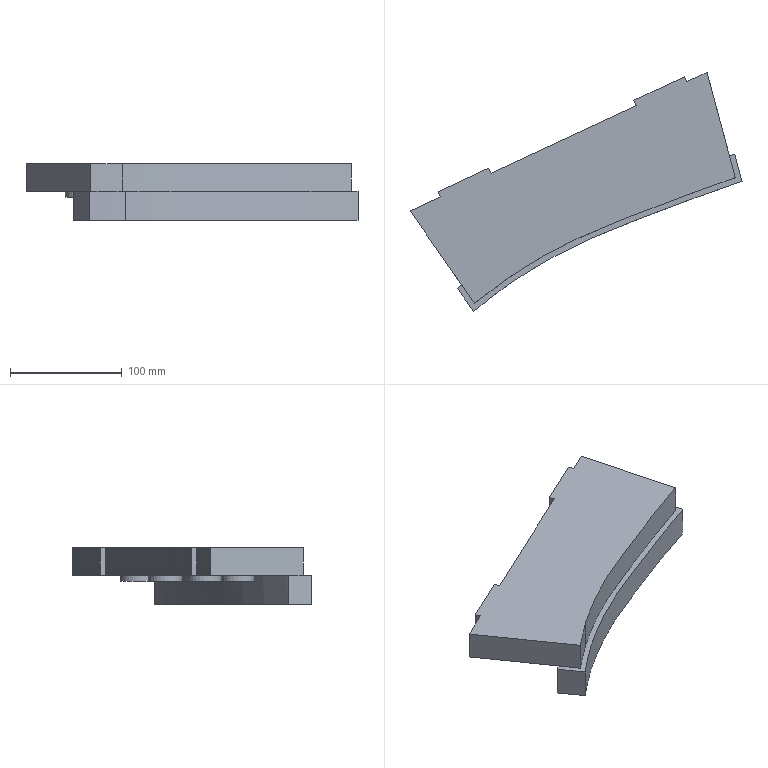Part | NX | features solid 2 | 1 solid | 32 faces | box 297.167 x 214.04 x 51 mm | volume 832670 mm3 | plane 22 | spline 5 | cylinder 5 | commonest cylinder face diameters 30 x5
STEP:
#1=CARTESIAN_POINT('',(-611.483,436.337,20.));
#2=VERTEX_POINT('',#1);
#3=CARTESIAN_POINT('',(-626.483,436.337,20.));
#4=DIRECTION('',(0.,0.,-1.));
#5=DIRECTION('',(1.,0.,0.));
#6=AXIS2_PLACEMENT_3D('',#3,#4,#5);
#7=CIRCLE('',#6,15.);
#8=EDGE_CURVE('',#2,#2,#7,.T.);
#9=ORIENTED_EDGE('',*,*,#8,.F.);
#10=EDGE_LOOP('',(#9));
#11=FACE_BOUND('',#10,.T.);
#12=CARTESIAN_POINT('',(-428.825,575.764,20.));
#13=VERTEX_POINT('',#12);
#14=CARTESIAN_POINT('',(-410.699,584.216,20.));
#15=VERTEX_POINT('',#14);
#16=CARTESIAN_POINT('',(-682.774,457.345,20.));
#17=DIRECTION('',(0.9063,0.4226,0.));
#18=VECTOR('',#17,1000.);
#19=LINE('',#16,#18);
#20=EDGE_CURVE('',#13,#15,#19,.T.);
#21=ORIENTED_EDGE('',*,*,#20,.T.);
#22=CARTESIAN_POINT('',(-390.647,509.382,20.));
#23=VERTEX_POINT('',#22);
#24=CARTESIAN_POINT('',(-381.309,474.533,20.));
#25=DIRECTION('',(0.2588,-0.9659,0.));
#26=VECTOR('',#25,1000.);
#27=LINE('',#24,#26);
#28=EDGE_CURVE('',#15,#23,#27,.T.);
#29=ORIENTED_EDGE('',*,*,#28,.T.);
#30=CARTESIAN_POINT('',(-630.157,393.945,20.));
#31=VERTEX_POINT('',#30);
#32=CARTESIAN_POINT('',(-630.157,393.945,20.));
#33=CARTESIAN_POINT('',(-625.863,397.477,20.));
#34=CARTESIAN_POINT('',(-617.15,404.382,20.));
#35=CARTESIAN_POINT('',(-603.765,414.343,20.));
#36=CARTESIAN_POINT('',(-589.743,423.494,20.));
#37=CARTESIAN_POINT('',(-570.825,435.215,20.));
#38=CARTESIAN_POINT('',(-546.501,448.639,20.));
#39=CARTESIAN_POINT('',(-516.021,462.462,20.));
#40=CARTESIAN_POINT('',(-484.84,474.648,20.));
#41=CARTESIAN_POINT('',(-453.543,486.499,20.));
#42=CARTESIAN_POINT('',(-422.261,498.4,20.));
#43=CARTESIAN_POINT('',(-401.243,505.881,20.));
#44=CARTESIAN_POINT('',(-390.647,509.382,20.));
#45=B_SPLINE_CURVE_WITH_KNOTS('',3,(#32,#33,#34,#35,#36,#37,#38,#39,#40,#41,#42,#43,#44),.UNSPECIFIED.,.F.,.F.,(4,1,1,1,1,1,1,1,1,1,4),(1.104,1.12,1.137,1.154,1.17,1.204,1.237,1.271,1.304,1.337,1.371),.UNSPECIFIED.);
#46=EDGE_CURVE('',#31,#23,#45,.T.);
#47=ORIENTED_EDGE('',*,*,#46,.F.);
#48=CARTESIAN_POINT('',(-676.574,460.236,20.));
#49=VERTEX_POINT('',#48);
#50=CARTESIAN_POINT('',(-593.778,341.99,20.));
#51=DIRECTION('',(0.5736,-0.8192,0.));
#52=VECTOR('',#51,1000.);
#53=LINE('',#50,#52);
#54=EDGE_CURVE('',#31,#49,#53,.F.);
#55=ORIENTED_EDGE('',*,*,#54,.T.);
#56=CARTESIAN_POINT('',(-649.385,472.915,20.));
#57=VERTEX_POINT('',#56);
#58=CARTESIAN_POINT('',(-682.774,457.345,20.));
#59=DIRECTION('',(0.9063,0.4226,0.));
#60=VECTOR('',#59,1000.);
#61=LINE('',#58,#60);
#62=EDGE_CURVE('',#49,#57,#61,.T.);
#63=ORIENTED_EDGE('',*,*,#62,.T.);
#64=CARTESIAN_POINT('',(-651.498,477.446,20.));
#65=VERTEX_POINT('',#64);
#66=CARTESIAN_POINT('',(-651.498,477.446,20.));
#67=DIRECTION('',(0.4226,-0.9063,0.));
#68=VECTOR('',#67,1000.);
#69=LINE('',#66,#68);
#70=EDGE_CURVE('',#65,#57,#69,.T.);
#71=ORIENTED_EDGE('',*,*,#70,.F.);
#72=CARTESIAN_POINT('',(-606.183,498.577,20.));
#73=VERTEX_POINT('',#72);
#74=CARTESIAN_POINT('',(-684.887,461.877,20.));
#75=DIRECTION('',(0.9063,0.4226,0.));
#76=VECTOR('',#75,1000.);
#77=LINE('',#74,#76);
#78=EDGE_CURVE('',#65,#73,#77,.T.);
#79=ORIENTED_EDGE('',*,*,#78,.T.);
#80=CARTESIAN_POINT('',(-604.07,494.046,20.));
#81=VERTEX_POINT('',#80);
#82=CARTESIAN_POINT('',(-606.183,498.577,20.));
#83=DIRECTION('',(0.4226,-0.9063,0.));
#84=VECTOR('',#83,1000.);
#85=LINE('',#82,#84);
#86=EDGE_CURVE('',#73,#81,#85,.T.);
#87=ORIENTED_EDGE('',*,*,#86,.T.);
#88=CARTESIAN_POINT('',(-474.14,554.633,20.));
#89=VERTEX_POINT('',#88);
#90=CARTESIAN_POINT('',(-682.774,457.345,20.));
#91=DIRECTION('',(0.9063,0.4226,0.));
#92=VECTOR('',#91,1000.);
#93=LINE('',#90,#92);
#94=EDGE_CURVE('',#81,#89,#93,.T.);
#95=ORIENTED_EDGE('',*,*,#94,.T.);
#96=CARTESIAN_POINT('',(-476.253,559.164,20.));
#97=VERTEX_POINT('',#96);
#98=CARTESIAN_POINT('',(-476.253,559.164,20.));
#99=DIRECTION('',(0.4226,-0.9063,0.));
#100=VECTOR('',#99,1000.);
#101=LINE('',#98,#100);
#102=EDGE_CURVE('',#97,#89,#101,.T.);
#103=ORIENTED_EDGE('',*,*,#102,.F.);
#104=CARTESIAN_POINT('',(-430.938,580.295,20.));
#105=VERTEX_POINT('',#104);
#106=CARTESIAN_POINT('',(-491.516,552.047,20.));
#107=DIRECTION('',(0.9063,0.4226,0.));
#108=VECTOR('',#107,1000.);
#109=LINE('',#106,#108);
#110=EDGE_CURVE('',#97,#105,#109,.T.);
#111=ORIENTED_EDGE('',*,*,#110,.T.);
#112=CARTESIAN_POINT('',(-430.938,580.295,20.));
#113=DIRECTION('',(0.4226,-0.9063,0.));
#114=VECTOR('',#113,1000.);
#115=LINE('',#112,#114);
#116=EDGE_CURVE('',#105,#13,#115,.T.);
#117=ORIENTED_EDGE('',*,*,#116,.T.);
#118=EDGE_LOOP('',(#21,#29,#47,#55,#63,#71,#79,#87,#95,#103,#111,#117));
#119=FACE_BOUND('',#118,.T.);
#120=CARTESIAN_POINT('',(-446.483,526.337,20.));
#121=VERTEX_POINT('',#120);
#122=CARTESIAN_POINT('',(-461.483,526.337,20.));
#123=DIRECTION('',(0.,0.,-1.));
#124=DIRECTION('',(1.,0.,0.));
#125=AXIS2_PLACEMENT_3D('',#122,#123,#124);
#126=CIRCLE('',#125,15.);
#127=EDGE_CURVE('',#121,#121,#126,.T.);
#128=ORIENTED_EDGE('',*,*,#127,.F.);
#129=EDGE_LOOP('',(#128));
#130=FACE_BOUND('',#129,.T.);
#131=CARTESIAN_POINT('',(-406.483,526.337,20.));
#132=VERTEX_POINT('',#131);
#133=CARTESIAN_POINT('',(-421.483,526.337,20.));
#134=DIRECTION('',(0.,0.,-1.));
#135=DIRECTION('',(1.,0.,0.));
#136=AXIS2_PLACEMENT_3D('',#133,#134,#135);
#137=CIRCLE('',#136,15.);
#138=EDGE_CURVE('',#132,#132,#137,.T.);
#139=ORIENTED_EDGE('',*,*,#138,.F.);
#140=EDGE_LOOP('',(#139));
#141=FACE_BOUND('',#140,.T.);
#142=CARTESIAN_POINT('',(-586.483,466.337,20.));
#143=VERTEX_POINT('',#142);
#144=CARTESIAN_POINT('',(-601.483,466.337,20.));
#145=DIRECTION('',(0.,0.,-1.));
#146=DIRECTION('',(1.,0.,0.));
#147=AXIS2_PLACEMENT_3D('',#144,#145,#146);
#148=CIRCLE('',#147,15.);
#149=EDGE_CURVE('',#143,#143,#148,.T.);
#150=ORIENTED_EDGE('',*,*,#149,.F.);
#151=EDGE_LOOP('',(#150));
#152=FACE_BOUND('',#151,.T.);
#153=CARTESIAN_POINT('',(-516.483,501.337,20.));
#154=VERTEX_POINT('',#153);
#155=CARTESIAN_POINT('',(-531.483,501.337,20.));
#156=DIRECTION('',(0.,0.,-1.));
#157=DIRECTION('',(1.,0.,0.));
#158=AXIS2_PLACEMENT_3D('',#155,#156,#157);
#159=CIRCLE('',#158,15.);
#160=EDGE_CURVE('',#154,#154,#159,.T.);
#161=ORIENTED_EDGE('',*,*,#160,.F.);
#162=EDGE_LOOP('',(#161));
#163=FACE_BOUND('',#162,.T.);
#164=CARTESIAN_POINT('',(-561.977,359.461,20.));
#165=DIRECTION('',(0.,0.,-1.));
#166=DIRECTION('',(-1.,0.,0.));
#167=AXIS2_PLACEMENT_3D('',#164,#165,#166);
#168=PLANE('',#167);
#169=ADVANCED_FACE('',(#11,#119,#130,#141,#152,#163),#168,.T.);
#170=CARTESIAN_POINT('',(-410.699,584.216,45.));
#171=VERTEX_POINT('',#170);
#172=CARTESIAN_POINT('',(-385.462,490.03,45.));
#173=VERTEX_POINT('',#172);
#174=CARTESIAN_POINT('',(-381.309,474.533,45.));
#175=DIRECTION('',(0.2588,-0.9659,0.));
#176=VECTOR('',#175,1000.);
#177=LINE('',#174,#176);
#178=EDGE_CURVE('',#171,#173,#177,.T.);
#179=ORIENTED_EDGE('',*,*,#178,.F.);
#180=CARTESIAN_POINT('',(-428.825,575.764,45.));
#181=VERTEX_POINT('',#180);
#182=CARTESIAN_POINT('',(-682.774,457.345,45.));
#183=DIRECTION('',(0.9063,0.4226,0.));
#184=VECTOR('',#183,1000.);
#185=LINE('',#182,#184);
#186=EDGE_CURVE('',#181,#171,#185,.T.);
#187=ORIENTED_EDGE('',*,*,#186,.F.);
#188=CARTESIAN_POINT('',(-430.938,580.295,45.));
#189=VERTEX_POINT('',#188);
#190=CARTESIAN_POINT('',(-430.938,580.295,45.));
#191=DIRECTION('',(0.4226,-0.9063,0.));
#192=VECTOR('',#191,1000.);
#193=LINE('',#190,#192);
#194=EDGE_CURVE('',#189,#181,#193,.T.);
#195=ORIENTED_EDGE('',*,*,#194,.F.);
#196=CARTESIAN_POINT('',(-476.253,559.164,45.));
#197=VERTEX_POINT('',#196);
#198=CARTESIAN_POINT('',(-491.516,552.047,45.));
#199=DIRECTION('',(0.9063,0.4226,0.));
#200=VECTOR('',#199,1000.);
#201=LINE('',#198,#200);
#202=EDGE_CURVE('',#197,#189,#201,.T.);
#203=ORIENTED_EDGE('',*,*,#202,.F.);
#204=CARTESIAN_POINT('',(-474.14,554.633,45.));
#205=VERTEX_POINT('',#204);
#206=CARTESIAN_POINT('',(-476.253,559.164,45.));
#207=DIRECTION('',(0.4226,-0.9063,0.));
#208=VECTOR('',#207,1000.);
#209=LINE('',#206,#208);
#210=EDGE_CURVE('',#197,#205,#209,.T.);
#211=ORIENTED_EDGE('',*,*,#210,.T.);
#212=CARTESIAN_POINT('',(-604.07,494.046,45.));
#213=VERTEX_POINT('',#212);
#214=CARTESIAN_POINT('',(-682.774,457.345,45.));
#215=DIRECTION('',(0.9063,0.4226,0.));
#216=VECTOR('',#215,1000.);
#217=LINE('',#214,#216);
#218=EDGE_CURVE('',#213,#205,#217,.T.);
#219=ORIENTED_EDGE('',*,*,#218,.F.);
#220=CARTESIAN_POINT('',(-606.183,498.577,45.));
#221=VERTEX_POINT('',#220);
#222=CARTESIAN_POINT('',(-606.183,498.577,45.));
#223=DIRECTION('',(0.4226,-0.9063,0.));
#224=VECTOR('',#223,1000.);
#225=LINE('',#222,#224);
#226=EDGE_CURVE('',#221,#213,#225,.T.);
#227=ORIENTED_EDGE('',*,*,#226,.F.);
#228=CARTESIAN_POINT('',(-651.498,477.446,45.));
#229=VERTEX_POINT('',#228);
#230=CARTESIAN_POINT('',(-684.887,461.877,45.));
#231=DIRECTION('',(0.9063,0.4226,0.));
#232=VECTOR('',#231,1000.);
#233=LINE('',#230,#232);
#234=EDGE_CURVE('',#229,#221,#233,.T.);
#235=ORIENTED_EDGE('',*,*,#234,.F.);
#236=CARTESIAN_POINT('',(-649.385,472.915,45.));
#237=VERTEX_POINT('',#236);
#238=CARTESIAN_POINT('',(-651.498,477.446,45.));
#239=DIRECTION('',(0.4226,-0.9063,0.));
#240=VECTOR('',#239,1000.);
#241=LINE('',#238,#240);
#242=EDGE_CURVE('',#229,#237,#241,.T.);
#243=ORIENTED_EDGE('',*,*,#242,.T.);
#244=CARTESIAN_POINT('',(-676.574,460.236,45.));
#245=VERTEX_POINT('',#244);
#246=CARTESIAN_POINT('',(-682.774,457.345,45.));
#247=DIRECTION('',(0.9063,0.4226,0.));
#248=VECTOR('',#247,1000.);
#249=LINE('',#246,#248);
#250=EDGE_CURVE('',#245,#237,#249,.T.);
#251=ORIENTED_EDGE('',*,*,#250,.F.);
#252=CARTESIAN_POINT('',(-618.649,377.51,45.));
#253=VERTEX_POINT('',#252);
#254=CARTESIAN_POINT('',(-593.778,341.99,45.));
#255=DIRECTION('',(0.5736,-0.8192,0.));
#256=VECTOR('',#255,1000.);
#257=LINE('',#254,#256);
#258=EDGE_CURVE('',#253,#245,#257,.F.);
#259=ORIENTED_EDGE('',*,*,#258,.F.);
#260=CARTESIAN_POINT('',(-590.38,399.095,45.));
#261=VERTEX_POINT('',#260);
#262=CARTESIAN_POINT('',(-590.38,399.095,45.));
#263=CARTESIAN_POINT('',(-592.782,397.416,45.));
#264=CARTESIAN_POINT('',(-597.653,393.932,45.));
#265=CARTESIAN_POINT('',(-607.128,386.839,45.));
#266=CARTESIAN_POINT('',(-614.087,381.289,45.));
#267=CARTESIAN_POINT('',(-618.649,377.51,45.));
#268=B_SPLINE_CURVE_WITH_KNOTS('',3,(#262,#263,#264,#265,#266,#267),.UNSPECIFIED.,.F.,.F.,(4,1,1,4),(-0.001177,0.2157,0.4325,0.8662),.UNSPECIFIED.);
#269=EDGE_CURVE('',#261,#253,#268,.T.);
#270=ORIENTED_EDGE('',*,*,#269,.F.);
#271=CARTESIAN_POINT('',(-385.462,490.03,45.));
#272=CARTESIAN_POINT('',(-403.254,484.121,45.));
#273=CARTESIAN_POINT('',(-429.525,474.262,45.));
#274=CARTESIAN_POINT('',(-464.312,461.014,45.));
#275=CARTESIAN_POINT('',(-490.467,451.058,45.));
#276=CARTESIAN_POINT('',(-516.53,440.426,45.));
#277=CARTESIAN_POINT('',(-542.098,428.317,45.));
#278=CARTESIAN_POINT('',(-562.642,416.758,45.));
#279=CARTESIAN_POINT('',(-578.61,406.867,45.));
#280=CARTESIAN_POINT('',(-586.513,401.689,45.));
#281=CARTESIAN_POINT('',(-590.38,399.095,45.));
#282=B_SPLINE_CURVE_WITH_KNOTS('',3,(#271,#272,#273,#274,#275,#276,#277,#278,#279,#280,#281),.UNSPECIFIED.,.F.,.F.,(4,1,1,1,1,1,1,1,4),(0.02066,0.2655,0.388,0.5104,0.6329,0.7553,0.8778,0.939,1.),.UNSPECIFIED.);
#283=EDGE_CURVE('',#173,#261,#282,.T.);
#284=ORIENTED_EDGE('',*,*,#283,.F.);
#285=EDGE_LOOP('',(#179,#187,#195,#203,#211,#219,#227,#235,#243,#251,#259,#270,#284));
#286=FACE_BOUND('',#285,.T.);
#287=CARTESIAN_POINT('',(-80.139,-794.984,45.));
#288=DIRECTION('',(0.,0.,1.));
#289=DIRECTION('',(1.,0.,0.));
#290=AXIS2_PLACEMENT_3D('',#287,#288,#289);
#291=PLANE('',#290);
#292=ADVANCED_FACE('',(#286),#291,.T.);
#293=ORIENTED_EDGE('',*,*,#178,.T.);
#294=CARTESIAN_POINT('',(-385.462,490.03,20.));
#295=VERTEX_POINT('',#294);
#296=CARTESIAN_POINT('',(-385.462,490.03,32.5));
#297=DIRECTION('',(0.,0.,1.));
#298=VECTOR('',#297,1000.);
#299=LINE('',#296,#298);
#300=EDGE_CURVE('',#295,#173,#299,.T.);
#301=ORIENTED_EDGE('',*,*,#300,.F.);
#302=CARTESIAN_POINT('',(-390.717,509.641,20.));
#303=DIRECTION('',(0.2588,-0.9659,0.));
#304=VECTOR('',#303,1000.);
#305=LINE('',#302,#304);
#306=EDGE_CURVE('',#23,#295,#305,.T.);
#307=ORIENTED_EDGE('',*,*,#306,.F.);
#308=ORIENTED_EDGE('',*,*,#28,.F.);
#309=CARTESIAN_POINT('',(-410.699,584.216,51.));
#310=DIRECTION('',(0.,0.,1.));
#311=VECTOR('',#310,1000.);
#312=LINE('',#309,#311);
#313=EDGE_CURVE('',#15,#171,#312,.T.);
#314=ORIENTED_EDGE('',*,*,#313,.T.);
#315=EDGE_LOOP('',(#293,#301,#307,#308,#314));
#316=FACE_BOUND('',#315,.T.);
#317=CARTESIAN_POINT('',(-381.309,474.533,20.));
#318=DIRECTION('',(-0.9659,-0.2588,0.));
#319=DIRECTION('',(0.2588,-0.9659,0.));
#320=AXIS2_PLACEMENT_3D('',#317,#318,#319);
#321=PLANE('',#320);
#322=ADVANCED_FACE('',(#316),#321,.F.);
#323=CARTESIAN_POINT('',(-618.649,377.51,20.));
#324=VERTEX_POINT('',#323);
#325=CARTESIAN_POINT('',(-618.649,377.51,32.5));
#326=DIRECTION('',(0.,0.,1.));
#327=VECTOR('',#326,1000.);
#328=LINE('',#325,#327);
#329=EDGE_CURVE('',#253,#324,#328,.F.);
#330=ORIENTED_EDGE('',*,*,#329,.F.);
#331=ORIENTED_EDGE('',*,*,#258,.T.);
#332=CARTESIAN_POINT('',(-676.574,460.236,51.));
#333=DIRECTION('',(0.,0.,-1.));
#334=VECTOR('',#333,1000.);
#335=LINE('',#332,#334);
#336=EDGE_CURVE('',#245,#49,#335,.T.);
#337=ORIENTED_EDGE('',*,*,#336,.T.);
#338=ORIENTED_EDGE('',*,*,#54,.F.);
#339=CARTESIAN_POINT('',(-593.778,341.99,20.));
#340=DIRECTION('',(0.5736,-0.8192,0.));
#341=VECTOR('',#340,1000.);
#342=LINE('',#339,#341);
#343=EDGE_CURVE('',#324,#31,#342,.F.);
#344=ORIENTED_EDGE('',*,*,#343,.F.);
#345=EDGE_LOOP('',(#330,#331,#337,#338,#344));
#346=FACE_BOUND('',#345,.T.);
#347=CARTESIAN_POINT('',(-593.778,341.99,45.));
#348=DIRECTION('',(-0.8192,-0.5736,0.));
#349=DIRECTION('',(0.5736,-0.8192,0.));
#350=AXIS2_PLACEMENT_3D('',#347,#348,#349);
#351=PLANE('',#350);
#352=ADVANCED_FACE('',(#346),#351,.T.);
#353=CARTESIAN_POINT('',(-590.38,399.095,20.));
#354=VERTEX_POINT('',#353);
#355=CARTESIAN_POINT('',(-385.462,490.03,20.));
#356=CARTESIAN_POINT('',(-403.254,484.121,20.));
#357=CARTESIAN_POINT('',(-429.525,474.262,20.));
#358=CARTESIAN_POINT('',(-464.312,461.014,20.));
#359=CARTESIAN_POINT('',(-490.467,451.058,20.));
#360=CARTESIAN_POINT('',(-516.53,440.426,20.));
#361=CARTESIAN_POINT('',(-542.098,428.317,20.));
#362=CARTESIAN_POINT('',(-562.642,416.758,20.));
#363=CARTESIAN_POINT('',(-578.61,406.867,20.));
#364=CARTESIAN_POINT('',(-586.513,401.689,20.));
#365=CARTESIAN_POINT('',(-590.38,399.095,20.));
#366=B_SPLINE_CURVE_WITH_KNOTS('',3,(#355,#356,#357,#358,#359,#360,#361,#362,#363,#364,#365),.UNSPECIFIED.,.F.,.F.,(4,1,1,1,1,1,1,1,4),(0.02066,0.2655,0.388,0.5104,0.6329,0.7553,0.8778,0.939,1.),.UNSPECIFIED.);
#367=EDGE_CURVE('',#295,#354,#366,.T.);
#368=ORIENTED_EDGE('',*,*,#367,.T.);
#369=CARTESIAN_POINT('',(-590.38,399.095,20.));
#370=CARTESIAN_POINT('',(-592.782,397.416,20.));
#371=CARTESIAN_POINT('',(-597.653,393.932,20.));
#372=CARTESIAN_POINT('',(-607.128,386.839,20.));
#373=CARTESIAN_POINT('',(-614.087,381.289,20.));
#374=CARTESIAN_POINT('',(-618.649,377.51,20.));
#375=B_SPLINE_CURVE_WITH_KNOTS('',3,(#369,#370,#371,#372,#373,#374),.UNSPECIFIED.,.F.,.F.,(4,1,1,4),(-0.001177,0.2157,0.4325,0.8662),.UNSPECIFIED.);
#376=EDGE_CURVE('',#354,#324,#375,.T.);
#377=ORIENTED_EDGE('',*,*,#376,.T.);
#378=ORIENTED_EDGE('',*,*,#343,.T.);
#379=CARTESIAN_POINT('',(-634.015,390.737,20.));
#380=VERTEX_POINT('',#379);
#381=CARTESIAN_POINT('',(-634.015,390.737,20.));
#382=CARTESIAN_POINT('',(-632.734,391.813,20.));
#383=CARTESIAN_POINT('',(-631.448,392.882,20.));
#384=CARTESIAN_POINT('',(-630.157,393.945,20.));
#385=B_SPLINE_CURVE_WITH_KNOTS('',3,(#381,#382,#383,#384),.UNSPECIFIED.,.F.,.F.,(4,4),(1.099,1.104),.UNSPECIFIED.);
#386=EDGE_CURVE('',#31,#380,#385,.F.);
#387=ORIENTED_EDGE('',*,*,#386,.T.);
#388=CARTESIAN_POINT('',(-619.617,370.176,20.));
#389=VERTEX_POINT('',#388);
#390=CARTESIAN_POINT('',(-619.617,370.176,20.));
#391=DIRECTION('',(0.5736,-0.8192,0.));
#392=VECTOR('',#391,1000.);
#393=LINE('',#390,#392);
#394=EDGE_CURVE('',#380,#389,#393,.T.);
#395=ORIENTED_EDGE('',*,*,#394,.T.);
#396=CARTESIAN_POINT('',(-587.555,394.969,20.));
#397=VERTEX_POINT('',#396);
#398=CARTESIAN_POINT('',(-587.555,394.969,20.));
#399=CARTESIAN_POINT('',(-598.633,387.227,20.));
#400=CARTESIAN_POINT('',(-609.306,378.914,20.));
#401=CARTESIAN_POINT('',(-619.617,370.176,20.));
#402=B_SPLINE_CURVE_WITH_KNOTS('',3,(#398,#399,#400,#401),.UNSPECIFIED.,.F.,.F.,(4,4),(0.8491,1.),.PIECEWISE_BEZIER_KNOTS.);
#403=EDGE_CURVE('',#389,#397,#402,.F.);
#404=ORIENTED_EDGE('',*,*,#403,.T.);
#405=CARTESIAN_POINT('',(-379.408,486.755,20.));
#406=VERTEX_POINT('',#405);
#407=CARTESIAN_POINT('',(-379.408,486.755,20.));
#408=CARTESIAN_POINT('',(-396.269,481.282,20.));
#409=CARTESIAN_POINT('',(-422.046,471.772,20.));
#410=CARTESIAN_POINT('',(-456.779,458.517,20.));
#411=CARTESIAN_POINT('',(-484.05,448.183,20.));
#412=CARTESIAN_POINT('',(-511.125,437.331,20.));
#413=CARTESIAN_POINT('',(-546.415,420.942,20.));
#414=CARTESIAN_POINT('',(-571.409,405.8,20.));
#415=CARTESIAN_POINT('',(-587.555,394.969,20.));
#416=B_SPLINE_CURVE_WITH_KNOTS('',3,(#407,#408,#409,#410,#411,#412,#413,#414,#415),.UNSPECIFIED.,.F.,.F.,(4,1,1,1,1,1,4),(0.,0.198,0.3065,0.415,0.5236,0.6321,0.8491),.UNSPECIFIED.);
#417=EDGE_CURVE('',#397,#406,#416,.F.);
#418=ORIENTED_EDGE('',*,*,#417,.T.);
#419=CARTESIAN_POINT('',(-385.887,510.936,20.));
#420=VERTEX_POINT('',#419);
#421=CARTESIAN_POINT('',(-385.887,510.936,20.));
#422=DIRECTION('',(-0.2588,0.9659,0.));
#423=VECTOR('',#422,1000.);
#424=LINE('',#421,#423);
#425=EDGE_CURVE('',#406,#420,#424,.T.);
#426=ORIENTED_EDGE('',*,*,#425,.T.);
#427=CARTESIAN_POINT('',(-634.015,390.737,20.));
#428=CARTESIAN_POINT('',(-623.724,399.378,20.));
#429=CARTESIAN_POINT('',(-613.022,407.671,20.));
#430=CARTESIAN_POINT('',(-601.876,415.461,20.));
#431=CARTESIAN_POINT('',(-601.745,415.552,20.));
#432=CARTESIAN_POINT('',(-601.614,415.642,20.));
#433=CARTESIAN_POINT('',(-601.482,415.731,20.));
#434=CARTESIAN_POINT('',(-584.696,426.991,20.));
#435=CARTESIAN_POINT('',(-558.325,442.982,20.));
#436=CARTESIAN_POINT('',(-520.945,460.334,20.));
#437=CARTESIAN_POINT('',(-492.999,471.527,20.));
#438=CARTESIAN_POINT('',(-465.644,481.892,20.));
#439=CARTESIAN_POINT('',(-430.564,495.278,20.));
#440=CARTESIAN_POINT('',(-403.706,505.189,20.));
#441=CARTESIAN_POINT('',(-385.887,510.936,20.));
#442=B_SPLINE_CURVE_WITH_KNOTS('',3,(#427,#428,#429,#430,#431,#432,#433,#434,#435,#436,#437,#438,#439,#440,#441),.UNSPECIFIED.,.F.,.F.,(4,3,3,1,1,1,1,1,4),(0.,0.1468,0.1485,0.365,0.4732,0.5815,0.6897,0.7979,1.),.UNSPECIFIED.);
#443=EDGE_CURVE('',#420,#23,#442,.F.);
#444=ORIENTED_EDGE('',*,*,#443,.T.);
#445=ORIENTED_EDGE('',*,*,#306,.T.);
#446=EDGE_LOOP('',(#368,#377,#378,#387,#395,#404,#418,#426,#444,#445));
#447=FACE_BOUND('',#446,.T.);
#448=CARTESIAN_POINT('',(-587.555,394.969,20.));
#449=DIRECTION('',(0.,0.,-1.));
#450=DIRECTION('',(-1.,0.,0.));
#451=AXIS2_PLACEMENT_3D('',#448,#449,#450);
#452=PLANE('',#451);
#453=ADVANCED_FACE('',(#447),#452,.F.);
#454=ORIENTED_EDGE('',*,*,#403,.F.);
#455=CARTESIAN_POINT('',(-619.617,370.176,-6.));
#456=VERTEX_POINT('',#455);
#457=CARTESIAN_POINT('',(-619.617,370.176,45.));
#458=DIRECTION('',(0.,0.,-1.));
#459=VECTOR('',#458,1000.);
#460=LINE('',#457,#459);
#461=EDGE_CURVE('',#389,#456,#460,.T.);
#462=ORIENTED_EDGE('',*,*,#461,.T.);
#463=CARTESIAN_POINT('',(-587.555,394.969,-6.));
#464=VERTEX_POINT('',#463);
#465=CARTESIAN_POINT('',(-587.555,394.969,-6.));
#466=CARTESIAN_POINT('',(-598.633,387.227,-6.));
#467=CARTESIAN_POINT('',(-609.306,378.914,-6.));
#468=CARTESIAN_POINT('',(-619.617,370.176,-6.));
#469=B_SPLINE_CURVE_WITH_KNOTS('',3,(#465,#466,#467,#468),.UNSPECIFIED.,.F.,.F.,(4,4),(0.8491,1.),.PIECEWISE_BEZIER_KNOTS.);
#470=EDGE_CURVE('',#464,#456,#469,.T.);
#471=ORIENTED_EDGE('',*,*,#470,.F.);
#472=CARTESIAN_POINT('',(-587.555,394.969,45.));
#473=DIRECTION('',(0.,0.,-1.));
#474=VECTOR('',#473,1000.);
#475=LINE('',#472,#474);
#476=EDGE_CURVE('',#397,#464,#475,.T.);
#477=ORIENTED_EDGE('',*,*,#476,.F.);
#478=EDGE_LOOP('',(#454,#462,#471,#477));
#479=FACE_BOUND('',#478,.T.);
#480=CARTESIAN_POINT('',(-587.555,394.969,20.));
#481=CARTESIAN_POINT('',(-587.555,394.969,-6.));
#482=CARTESIAN_POINT('',(-598.633,387.227,20.));
#483=CARTESIAN_POINT('',(-598.633,387.227,-6.));
#484=CARTESIAN_POINT('',(-609.306,378.914,20.));
#485=CARTESIAN_POINT('',(-609.306,378.914,-6.));
#486=CARTESIAN_POINT('',(-619.617,370.176,20.));
#487=CARTESIAN_POINT('',(-619.617,370.176,-6.));
#488=B_SPLINE_SURFACE_WITH_KNOTS('',3,1,((#480,#481),(#482,#483),(#484,#485),(#486,#487)),.SURF_OF_LINEAR_EXTRUSION.,.F.,.F.,.F.,(4,4),(2,2),(0.8491,1.),(0.,1.),.PIECEWISE_BEZIER_KNOTS.);
#489=ADVANCED_FACE('',(#479),#488,.T.);
#490=CARTESIAN_POINT('',(-379.408,486.755,-6.));
#491=VERTEX_POINT('',#490);
#492=CARTESIAN_POINT('',(-379.408,486.755,45.));
#493=DIRECTION('',(0.,0.,-1.));
#494=VECTOR('',#493,1000.);
#495=LINE('',#492,#494);
#496=EDGE_CURVE('',#406,#491,#495,.T.);
#497=ORIENTED_EDGE('',*,*,#496,.F.);
#498=ORIENTED_EDGE('',*,*,#417,.F.);
#499=ORIENTED_EDGE('',*,*,#476,.T.);
#500=CARTESIAN_POINT('',(-379.408,486.755,-6.));
#501=CARTESIAN_POINT('',(-396.269,481.282,-6.));
#502=CARTESIAN_POINT('',(-422.046,471.772,-6.));
#503=CARTESIAN_POINT('',(-456.779,458.517,-6.));
#504=CARTESIAN_POINT('',(-484.05,448.183,-6.));
#505=CARTESIAN_POINT('',(-511.125,437.331,-6.));
#506=CARTESIAN_POINT('',(-546.415,420.942,-6.));
#507=CARTESIAN_POINT('',(-571.409,405.8,-6.));
#508=CARTESIAN_POINT('',(-587.555,394.969,-6.));
#509=B_SPLINE_CURVE_WITH_KNOTS('',3,(#500,#501,#502,#503,#504,#505,#506,#507,#508),.UNSPECIFIED.,.F.,.F.,(4,1,1,1,1,1,4),(0.,0.198,0.3065,0.415,0.5236,0.6321,0.8491),.UNSPECIFIED.);
#510=EDGE_CURVE('',#491,#464,#509,.T.);
#511=ORIENTED_EDGE('',*,*,#510,.F.);
#512=EDGE_LOOP('',(#497,#498,#499,#511));
#513=FACE_BOUND('',#512,.T.);
#514=CARTESIAN_POINT('',(-379.408,486.755,20.));
#515=CARTESIAN_POINT('',(-379.408,486.755,-6.));
#516=CARTESIAN_POINT('',(-397.486,480.886,20.));
#517=CARTESIAN_POINT('',(-397.486,480.886,-6.));
#518=CARTESIAN_POINT('',(-424.239,470.933,20.));
#519=CARTESIAN_POINT('',(-424.239,470.933,-6.));
#520=CARTESIAN_POINT('',(-459.771,457.384,20.));
#521=CARTESIAN_POINT('',(-459.771,457.384,-6.));
#522=CARTESIAN_POINT('',(-486.438,447.26,20.));
#523=CARTESIAN_POINT('',(-486.438,447.26,-6.));
#524=CARTESIAN_POINT('',(-512.886,436.564,20.));
#525=CARTESIAN_POINT('',(-512.886,436.564,-6.));
#526=CARTESIAN_POINT('',(-547.338,420.401,20.));
#527=CARTESIAN_POINT('',(-547.338,420.401,-6.));
#528=CARTESIAN_POINT('',(-571.763,405.563,20.));
#529=CARTESIAN_POINT('',(-571.763,405.563,-6.));
#530=CARTESIAN_POINT('',(-587.555,394.969,20.));
#531=CARTESIAN_POINT('',(-587.555,394.969,-6.));
#532=B_SPLINE_SURFACE_WITH_KNOTS('',3,1,((#514,#515),(#516,#517),(#518,#519),(#520,#521),(#522,#523),(#524,#525),(#526,#527),(#528,#529),(#530,#531)),.SURF_OF_LINEAR_EXTRUSION.,.F.,.F.,.F.,(4,1,1,1,1,1,4),(2,2),(0.,0.2123,0.3184,0.4246,0.5307,0.6368,0.8491),(0.,1.),.UNSPECIFIED.);
#533=ADVANCED_FACE('',(#513),#532,.T.);
#534=ORIENTED_EDGE('',*,*,#269,.T.);
#535=ORIENTED_EDGE('',*,*,#329,.T.);
#536=ORIENTED_EDGE('',*,*,#376,.F.);
#537=CARTESIAN_POINT('',(-590.38,399.095,32.5));
#538=DIRECTION('',(0.,0.,1.));
#539=VECTOR('',#538,1000.);
#540=LINE('',#537,#539);
#541=EDGE_CURVE('',#354,#261,#540,.T.);
#542=ORIENTED_EDGE('',*,*,#541,.T.);
#543=EDGE_LOOP('',(#534,#535,#536,#542));
#544=FACE_BOUND('',#543,.T.);
#545=CARTESIAN_POINT('',(-590.38,399.095,20.));
#546=CARTESIAN_POINT('',(-590.38,399.095,45.));
#547=CARTESIAN_POINT('',(-592.782,397.416,20.));
#548=CARTESIAN_POINT('',(-592.782,397.416,45.));
#549=CARTESIAN_POINT('',(-597.653,393.932,20.));
#550=CARTESIAN_POINT('',(-597.653,393.932,45.));
#551=CARTESIAN_POINT('',(-607.128,386.839,20.));
#552=CARTESIAN_POINT('',(-607.128,386.839,45.));
#553=CARTESIAN_POINT('',(-614.087,381.289,20.));
#554=CARTESIAN_POINT('',(-614.087,381.289,45.));
#555=CARTESIAN_POINT('',(-618.649,377.51,20.));
#556=CARTESIAN_POINT('',(-618.649,377.51,45.));
#557=B_SPLINE_SURFACE_WITH_KNOTS('',3,1,((#545,#546),(#547,#548),(#549,#550),(#551,#552),(#553,#554),(#555,#556)),.SURF_OF_LINEAR_EXTRUSION.,.F.,.F.,.F.,(4,1,1,4),(2,2),(-0.001177,0.2157,0.4325,0.8662),(0.,1.),.UNSPECIFIED.);
#558=ADVANCED_FACE('',(#544),#557,.F.);
#559=ORIENTED_EDGE('',*,*,#367,.F.);
#560=ORIENTED_EDGE('',*,*,#300,.T.);
#561=ORIENTED_EDGE('',*,*,#283,.T.);
#562=ORIENTED_EDGE('',*,*,#541,.F.);
#563=EDGE_LOOP('',(#559,#560,#561,#562));
#564=FACE_BOUND('',#563,.T.);
#565=CARTESIAN_POINT('',(-385.462,490.03,20.));
#566=CARTESIAN_POINT('',(-385.462,490.03,45.));
#567=CARTESIAN_POINT('',(-403.254,484.121,20.));
#568=CARTESIAN_POINT('',(-403.254,484.121,45.));
#569=CARTESIAN_POINT('',(-429.525,474.262,20.));
#570=CARTESIAN_POINT('',(-429.525,474.262,45.));
#571=CARTESIAN_POINT('',(-464.312,461.014,20.));
#572=CARTESIAN_POINT('',(-464.312,461.014,45.));
#573=CARTESIAN_POINT('',(-490.467,451.058,20.));
#574=CARTESIAN_POINT('',(-490.467,451.058,45.));
#575=CARTESIAN_POINT('',(-516.53,440.426,20.));
#576=CARTESIAN_POINT('',(-516.53,440.426,45.));
#577=CARTESIAN_POINT('',(-542.098,428.317,20.));
#578=CARTESIAN_POINT('',(-542.098,428.317,45.));
#579=CARTESIAN_POINT('',(-562.642,416.758,20.));
#580=CARTESIAN_POINT('',(-562.642,416.758,45.));
#581=CARTESIAN_POINT('',(-578.61,406.867,20.));
#582=CARTESIAN_POINT('',(-578.61,406.867,45.));
#583=CARTESIAN_POINT('',(-586.513,401.689,20.));
#584=CARTESIAN_POINT('',(-586.513,401.689,45.));
#585=CARTESIAN_POINT('',(-590.38,399.095,20.));
#586=CARTESIAN_POINT('',(-590.38,399.095,45.));
#587=B_SPLINE_SURFACE_WITH_KNOTS('',3,1,((#565,#566),(#567,#568),(#569,#570),(#571,#572),(#573,#574),(#575,#576),(#577,#578),(#579,#580),(#581,#582),(#583,#584),(#585,#586)),.SURF_OF_LINEAR_EXTRUSION.,.F.,.F.,.F.,(4,1,1,1,1,1,1,1,4),(2,2),(0.02066,0.2655,0.388,0.5104,0.6329,0.7553,0.8778,0.939,1.),(0.,1.),.UNSPECIFIED.);
#588=ADVANCED_FACE('',(#564),#587,.F.);
#589=ORIENTED_EDGE('',*,*,#46,.T.);
#590=ORIENTED_EDGE('',*,*,#443,.F.);
#591=CARTESIAN_POINT('',(-385.887,510.936,-6.));
#592=VERTEX_POINT('',#591);
#593=CARTESIAN_POINT('',(-385.887,510.936,45.));
#594=DIRECTION('',(0.,0.,-1.));
#595=VECTOR('',#594,1000.);
#596=LINE('',#593,#595);
#597=EDGE_CURVE('',#420,#592,#596,.T.);
#598=ORIENTED_EDGE('',*,*,#597,.T.);
#599=CARTESIAN_POINT('',(-634.015,390.737,-6.));
#600=VERTEX_POINT('',#599);
#601=CARTESIAN_POINT('',(-634.015,390.737,-6.));
#602=CARTESIAN_POINT('',(-623.724,399.378,-6.));
#603=CARTESIAN_POINT('',(-613.022,407.671,-6.));
#604=CARTESIAN_POINT('',(-601.876,415.461,-6.));
#605=CARTESIAN_POINT('',(-601.745,415.552,-6.));
#606=CARTESIAN_POINT('',(-601.614,415.642,-6.));
#607=CARTESIAN_POINT('',(-601.482,415.731,-6.));
#608=CARTESIAN_POINT('',(-584.696,426.991,-6.));
#609=CARTESIAN_POINT('',(-558.325,442.982,-6.));
#610=CARTESIAN_POINT('',(-520.945,460.334,-6.));
#611=CARTESIAN_POINT('',(-492.999,471.527,-6.));
#612=CARTESIAN_POINT('',(-465.644,481.892,-6.));
#613=CARTESIAN_POINT('',(-430.564,495.278,-6.));
#614=CARTESIAN_POINT('',(-403.706,505.189,-6.));
#615=CARTESIAN_POINT('',(-385.887,510.936,-6.));
#616=B_SPLINE_CURVE_WITH_KNOTS('',3,(#601,#602,#603,#604,#605,#606,#607,#608,#609,#610,#611,#612,#613,#614,#615),.UNSPECIFIED.,.F.,.F.,(4,3,3,1,1,1,1,1,4),(0.,0.1468,0.1485,0.365,0.4732,0.5815,0.6897,0.7979,1.),.UNSPECIFIED.);
#617=EDGE_CURVE('',#600,#592,#616,.T.);
#618=ORIENTED_EDGE('',*,*,#617,.F.);
#619=CARTESIAN_POINT('',(-634.015,390.737,45.));
#620=DIRECTION('',(0.,0.,-1.));
#621=VECTOR('',#620,1000.);
#622=LINE('',#619,#621);
#623=EDGE_CURVE('',#380,#600,#622,.T.);
#624=ORIENTED_EDGE('',*,*,#623,.F.);
#625=ORIENTED_EDGE('',*,*,#386,.F.);
#626=EDGE_LOOP('',(#589,#590,#598,#618,#624,#625));
#627=FACE_BOUND('',#626,.T.);
#628=CARTESIAN_POINT('',(-634.015,390.737,20.));
#629=CARTESIAN_POINT('',(-634.015,390.737,-6.));
#630=CARTESIAN_POINT('',(-629.633,394.417,20.));
#631=CARTESIAN_POINT('',(-629.633,394.417,-6.));
#632=CARTESIAN_POINT('',(-620.718,401.645,20.));
#633=CARTESIAN_POINT('',(-620.718,401.645,-6.));
#634=CARTESIAN_POINT('',(-609.192,410.33,20.));
#635=CARTESIAN_POINT('',(-609.192,410.33,-6.));
#636=CARTESIAN_POINT('',(-599.725,416.965,20.));
#637=CARTESIAN_POINT('',(-599.725,416.965,-6.));
#638=CARTESIAN_POINT('',(-589.886,423.364,20.));
#639=CARTESIAN_POINT('',(-589.886,423.364,-6.));
#640=CARTESIAN_POINT('',(-572.439,434.305,20.));
#641=CARTESIAN_POINT('',(-572.439,434.305,-6.));
#642=CARTESIAN_POINT('',(-546.472,448.726,20.));
#643=CARTESIAN_POINT('',(-546.472,448.726,-6.));
#644=CARTESIAN_POINT('',(-513.965,463.338,20.));
#645=CARTESIAN_POINT('',(-513.965,463.338,-6.));
#646=CARTESIAN_POINT('',(-481.898,475.756,20.));
#647=CARTESIAN_POINT('',(-481.898,475.756,-6.));
#648=CARTESIAN_POINT('',(-450.542,487.649,20.));
#649=CARTESIAN_POINT('',(-450.542,487.649,-6.));
#650=CARTESIAN_POINT('',(-418.718,499.724,20.));
#651=CARTESIAN_POINT('',(-418.718,499.724,-6.));
#652=CARTESIAN_POINT('',(-396.91,507.381,20.));
#653=CARTESIAN_POINT('',(-396.91,507.381,-6.));
#654=CARTESIAN_POINT('',(-385.887,510.936,20.));
#655=CARTESIAN_POINT('',(-385.887,510.936,-6.));
#656=B_SPLINE_SURFACE_WITH_KNOTS('',3,1,((#628,#629),(#630,#631),(#632,#633),(#634,#635),(#636,#637),(#638,#639),(#640,#641),(#642,#643),(#644,#645),(#646,#647),(#648,#649),(#650,#651),(#652,#653),(#654,#655)),.SURF_OF_LINEAR_EXTRUSION.,.F.,.F.,.F.,(4,1,1,1,1,1,1,1,1,1,1,4),(2,2),(0.,0.0625,0.125,0.1562,0.1875,0.25,0.375,0.5,0.625,0.75,0.875,1.),(0.,1.),.UNSPECIFIED.);
#657=ADVANCED_FACE('',(#627),#656,.T.);
#658=ORIENTED_EDGE('',*,*,#394,.F.);
#659=ORIENTED_EDGE('',*,*,#623,.T.);
#660=CARTESIAN_POINT('',(-619.617,370.176,-6.));
#661=DIRECTION('',(-0.5736,0.8192,0.));
#662=VECTOR('',#661,1000.);
#663=LINE('',#660,#662);
#664=EDGE_CURVE('',#456,#600,#663,.T.);
#665=ORIENTED_EDGE('',*,*,#664,.F.);
#666=ORIENTED_EDGE('',*,*,#461,.F.);
#667=EDGE_LOOP('',(#658,#659,#665,#666));
#668=FACE_BOUND('',#667,.T.);
#669=CARTESIAN_POINT('',(-634.015,390.737,51.));
#670=DIRECTION('',(-0.8192,-0.5736,0.));
#671=DIRECTION('',(0.5736,-0.8192,0.));
#672=AXIS2_PLACEMENT_3D('',#669,#670,#671);
#673=PLANE('',#672);
#674=ADVANCED_FACE('',(#668),#673,.T.);
#675=ORIENTED_EDGE('',*,*,#597,.F.);
#676=ORIENTED_EDGE('',*,*,#425,.F.);
#677=ORIENTED_EDGE('',*,*,#496,.T.);
#678=CARTESIAN_POINT('',(-385.887,510.936,-6.));
#679=DIRECTION('',(0.2588,-0.9659,0.));
#680=VECTOR('',#679,1000.);
#681=LINE('',#678,#680);
#682=EDGE_CURVE('',#592,#491,#681,.T.);
#683=ORIENTED_EDGE('',*,*,#682,.F.);
#684=EDGE_LOOP('',(#675,#676,#677,#683));
#685=FACE_BOUND('',#684,.T.);
#686=CARTESIAN_POINT('',(-385.887,510.936,51.));
#687=DIRECTION('',(-0.9659,-0.2588,0.));
#688=DIRECTION('',(0.2588,-0.9659,0.));
#689=AXIS2_PLACEMENT_3D('',#686,#687,#688);
#690=PLANE('',#689);
#691=ADVANCED_FACE('',(#685),#690,.F.);
#692=ORIENTED_EDGE('',*,*,#617,.T.);
#693=ORIENTED_EDGE('',*,*,#682,.T.);
#694=ORIENTED_EDGE('',*,*,#510,.T.);
#695=ORIENTED_EDGE('',*,*,#470,.T.);
#696=ORIENTED_EDGE('',*,*,#664,.T.);
#697=EDGE_LOOP('',(#692,#693,#694,#695,#696));
#698=FACE_BOUND('',#697,.T.);
#699=CARTESIAN_POINT('',(-514.038,462.972,-6.));
#700=DIRECTION('',(0.,0.,1.));
#701=DIRECTION('',(1.,0.,0.));
#702=AXIS2_PLACEMENT_3D('',#699,#700,#701);
#703=PLANE('',#702);
#704=ADVANCED_FACE('',(#698),#703,.F.);
#705=CARTESIAN_POINT('',(-428.825,575.764,51.));
#706=DIRECTION('',(0.,0.,1.));
#707=VECTOR('',#706,1000.);
#708=LINE('',#705,#707);
#709=EDGE_CURVE('',#13,#181,#708,.T.);
#710=ORIENTED_EDGE('',*,*,#709,.T.);
#711=ORIENTED_EDGE('',*,*,#186,.T.);
#712=ORIENTED_EDGE('',*,*,#313,.F.);
#713=ORIENTED_EDGE('',*,*,#20,.F.);
#714=EDGE_LOOP('',(#710,#711,#712,#713));
#715=FACE_BOUND('',#714,.T.);
#716=CARTESIAN_POINT('',(-682.774,457.345,51.));
#717=DIRECTION('',(-0.4226,0.9063,0.));
#718=DIRECTION('',(-0.9063,-0.4226,0.));
#719=AXIS2_PLACEMENT_3D('',#716,#717,#718);
#720=PLANE('',#719);
#721=ADVANCED_FACE('',(#715),#720,.T.);
#722=CARTESIAN_POINT('',(-474.14,554.633,51.));
#723=DIRECTION('',(0.,0.,-1.));
#724=VECTOR('',#723,1000.);
#725=LINE('',#722,#724);
#726=EDGE_CURVE('',#205,#89,#725,.T.);
#727=ORIENTED_EDGE('',*,*,#726,.T.);
#728=ORIENTED_EDGE('',*,*,#94,.F.);
#729=CARTESIAN_POINT('',(-604.07,494.046,51.));
#730=DIRECTION('',(0.,0.,1.));
#731=VECTOR('',#730,1000.);
#732=LINE('',#729,#731);
#733=EDGE_CURVE('',#81,#213,#732,.T.);
#734=ORIENTED_EDGE('',*,*,#733,.T.);
#735=ORIENTED_EDGE('',*,*,#218,.T.);
#736=EDGE_LOOP('',(#727,#728,#734,#735));
#737=FACE_BOUND('',#736,.T.);
#738=CARTESIAN_POINT('',(-682.774,457.345,51.));
#739=DIRECTION('',(-0.4226,0.9063,0.));
#740=DIRECTION('',(-0.9063,-0.4226,0.));
#741=AXIS2_PLACEMENT_3D('',#738,#739,#740);
#742=PLANE('',#741);
#743=ADVANCED_FACE('',(#737),#742,.T.);
#744=CARTESIAN_POINT('',(-649.385,472.915,51.));
#745=DIRECTION('',(0.,0.,-1.));
#746=VECTOR('',#745,1000.);
#747=LINE('',#744,#746);
#748=EDGE_CURVE('',#237,#57,#747,.T.);
#749=ORIENTED_EDGE('',*,*,#748,.T.);
#750=ORIENTED_EDGE('',*,*,#62,.F.);
#751=ORIENTED_EDGE('',*,*,#336,.F.);
#752=ORIENTED_EDGE('',*,*,#250,.T.);
#753=EDGE_LOOP('',(#749,#750,#751,#752));
#754=FACE_BOUND('',#753,.T.);
#755=CARTESIAN_POINT('',(-682.774,457.345,51.));
#756=DIRECTION('',(-0.4226,0.9063,0.));
#757=DIRECTION('',(-0.9063,-0.4226,0.));
#758=AXIS2_PLACEMENT_3D('',#755,#756,#757);
#759=PLANE('',#758);
#760=ADVANCED_FACE('',(#754),#759,.T.);
#761=ORIENTED_EDGE('',*,*,#160,.T.);
#762=EDGE_LOOP('',(#761));
#763=FACE_BOUND('',#762,.T.);
#764=CARTESIAN_POINT('',(-516.483,501.337,15.));
#765=VERTEX_POINT('',#764);
#766=CARTESIAN_POINT('',(-531.483,501.337,15.));
#767=DIRECTION('',(0.,0.,-1.));
#768=DIRECTION('',(1.,0.,0.));
#769=AXIS2_PLACEMENT_3D('',#766,#767,#768);
#770=CIRCLE('',#769,15.);
#771=EDGE_CURVE('',#765,#765,#770,.T.);
#772=ORIENTED_EDGE('',*,*,#771,.F.);
#773=EDGE_LOOP('',(#772));
#774=FACE_BOUND('',#773,.T.);
#775=CARTESIAN_POINT('',(-531.483,501.337,20.));
#776=DIRECTION('',(0.,0.,-1.));
#777=DIRECTION('',(-1.,0.,0.));
#778=AXIS2_PLACEMENT_3D('',#775,#776,#777);
#779=CYLINDRICAL_SURFACE('',#778,15.);
#780=ADVANCED_FACE('',(#763,#774),#779,.T.);
#781=ORIENTED_EDGE('',*,*,#771,.T.);
#782=EDGE_LOOP('',(#781));
#783=FACE_BOUND('',#782,.T.);
#784=CARTESIAN_POINT('',(-531.483,501.337,15.));
#785=DIRECTION('',(0.,0.,-1.));
#786=DIRECTION('',(-1.,0.,0.));
#787=AXIS2_PLACEMENT_3D('',#784,#785,#786);
#788=PLANE('',#787);
#789=ADVANCED_FACE('',(#783),#788,.T.);
#790=ORIENTED_EDGE('',*,*,#138,.T.);
#791=EDGE_LOOP('',(#790));
#792=FACE_BOUND('',#791,.T.);
#793=CARTESIAN_POINT('',(-406.483,526.337,15.));
#794=VERTEX_POINT('',#793);
#795=CARTESIAN_POINT('',(-421.483,526.337,15.));
#796=DIRECTION('',(0.,0.,-1.));
#797=DIRECTION('',(1.,0.,0.));
#798=AXIS2_PLACEMENT_3D('',#795,#796,#797);
#799=CIRCLE('',#798,15.);
#800=EDGE_CURVE('',#794,#794,#799,.T.);
#801=ORIENTED_EDGE('',*,*,#800,.F.);
#802=EDGE_LOOP('',(#801));
#803=FACE_BOUND('',#802,.T.);
#804=CARTESIAN_POINT('',(-421.483,526.337,20.));
#805=DIRECTION('',(0.,0.,-1.));
#806=DIRECTION('',(-1.,0.,0.));
#807=AXIS2_PLACEMENT_3D('',#804,#805,#806);
#808=CYLINDRICAL_SURFACE('',#807,15.);
#809=ADVANCED_FACE('',(#792,#803),#808,.T.);
#810=ORIENTED_EDGE('',*,*,#800,.T.);
#811=EDGE_LOOP('',(#810));
#812=FACE_BOUND('',#811,.T.);
#813=CARTESIAN_POINT('',(-421.483,526.337,15.));
#814=DIRECTION('',(0.,0.,-1.));
#815=DIRECTION('',(-1.,0.,0.));
#816=AXIS2_PLACEMENT_3D('',#813,#814,#815);
#817=PLANE('',#816);
#818=ADVANCED_FACE('',(#812),#817,.T.);
#819=ORIENTED_EDGE('',*,*,#8,.T.);
#820=EDGE_LOOP('',(#819));
#821=FACE_BOUND('',#820,.T.);
#822=CARTESIAN_POINT('',(-611.483,436.337,15.));
#823=VERTEX_POINT('',#822);
#824=CARTESIAN_POINT('',(-626.483,436.337,15.));
#825=DIRECTION('',(0.,0.,-1.));
#826=DIRECTION('',(1.,0.,0.));
#827=AXIS2_PLACEMENT_3D('',#824,#825,#826);
#828=CIRCLE('',#827,15.);
#829=EDGE_CURVE('',#823,#823,#828,.T.);
#830=ORIENTED_EDGE('',*,*,#829,.F.);
#831=EDGE_LOOP('',(#830));
#832=FACE_BOUND('',#831,.T.);
#833=CARTESIAN_POINT('',(-626.483,436.337,20.));
#834=DIRECTION('',(0.,0.,-1.));
#835=DIRECTION('',(-1.,0.,0.));
#836=AXIS2_PLACEMENT_3D('',#833,#834,#835);
#837=CYLINDRICAL_SURFACE('',#836,15.);
#838=ADVANCED_FACE('',(#821,#832),#837,.T.);
#839=ORIENTED_EDGE('',*,*,#829,.T.);
#840=EDGE_LOOP('',(#839));
#841=FACE_BOUND('',#840,.T.);
#842=CARTESIAN_POINT('',(-626.483,436.337,15.));
#843=DIRECTION('',(0.,0.,-1.));
#844=DIRECTION('',(-1.,0.,0.));
#845=AXIS2_PLACEMENT_3D('',#842,#843,#844);
#846=PLANE('',#845);
#847=ADVANCED_FACE('',(#841),#846,.T.);
#848=ORIENTED_EDGE('',*,*,#149,.T.);
#849=EDGE_LOOP('',(#848));
#850=FACE_BOUND('',#849,.T.);
#851=CARTESIAN_POINT('',(-586.483,466.337,15.));
#852=VERTEX_POINT('',#851);
#853=CARTESIAN_POINT('',(-601.483,466.337,15.));
#854=DIRECTION('',(0.,0.,-1.));
#855=DIRECTION('',(1.,0.,0.));
#856=AXIS2_PLACEMENT_3D('',#853,#854,#855);
#857=CIRCLE('',#856,15.);
#858=EDGE_CURVE('',#852,#852,#857,.T.);
#859=ORIENTED_EDGE('',*,*,#858,.F.);
#860=EDGE_LOOP('',(#859));
#861=FACE_BOUND('',#860,.T.);
#862=CARTESIAN_POINT('',(-601.483,466.337,20.));
#863=DIRECTION('',(0.,0.,-1.));
#864=DIRECTION('',(-1.,0.,0.));
#865=AXIS2_PLACEMENT_3D('',#862,#863,#864);
#866=CYLINDRICAL_SURFACE('',#865,15.);
#867=ADVANCED_FACE('',(#850,#861),#866,.T.);
#868=ORIENTED_EDGE('',*,*,#858,.T.);
#869=EDGE_LOOP('',(#868));
#870=FACE_BOUND('',#869,.T.);
#871=CARTESIAN_POINT('',(-601.483,466.337,15.));
#872=DIRECTION('',(0.,0.,-1.));
#873=DIRECTION('',(-1.,0.,0.));
#874=AXIS2_PLACEMENT_3D('',#871,#872,#873);
#875=PLANE('',#874);
#876=ADVANCED_FACE('',(#870),#875,.T.);
#877=ORIENTED_EDGE('',*,*,#127,.T.);
#878=EDGE_LOOP('',(#877));
#879=FACE_BOUND('',#878,.T.);
#880=CARTESIAN_POINT('',(-446.483,526.337,15.));
#881=VERTEX_POINT('',#880);
#882=CARTESIAN_POINT('',(-461.483,526.337,15.));
#883=DIRECTION('',(0.,0.,-1.));
#884=DIRECTION('',(1.,0.,0.));
#885=AXIS2_PLACEMENT_3D('',#882,#883,#884);
#886=CIRCLE('',#885,15.);
#887=EDGE_CURVE('',#881,#881,#886,.T.);
#888=ORIENTED_EDGE('',*,*,#887,.F.);
#889=EDGE_LOOP('',(#888));
#890=FACE_BOUND('',#889,.T.);
#891=CARTESIAN_POINT('',(-461.483,526.337,20.));
#892=DIRECTION('',(0.,0.,-1.));
#893=DIRECTION('',(-1.,0.,0.));
#894=AXIS2_PLACEMENT_3D('',#891,#892,#893);
#895=CYLINDRICAL_SURFACE('',#894,15.);
#896=ADVANCED_FACE('',(#879,#890),#895,.T.);
#897=ORIENTED_EDGE('',*,*,#887,.T.);
#898=EDGE_LOOP('',(#897));
#899=FACE_BOUND('',#898,.T.);
#900=CARTESIAN_POINT('',(-461.483,526.337,15.));
#901=DIRECTION('',(0.,0.,-1.));
#902=DIRECTION('',(-1.,0.,0.));
#903=AXIS2_PLACEMENT_3D('',#900,#901,#902);
#904=PLANE('',#903);
#905=ADVANCED_FACE('',(#899),#904,.T.);
#906=ORIENTED_EDGE('',*,*,#733,.F.);
#907=ORIENTED_EDGE('',*,*,#86,.F.);
#908=CARTESIAN_POINT('',(-606.183,498.577,51.));
#909=DIRECTION('',(0.,0.,1.));
#910=VECTOR('',#909,1000.);
#911=LINE('',#908,#910);
#912=EDGE_CURVE('',#73,#221,#911,.T.);
#913=ORIENTED_EDGE('',*,*,#912,.T.);
#914=ORIENTED_EDGE('',*,*,#226,.T.);
#915=EDGE_LOOP('',(#906,#907,#913,#914));
#916=FACE_BOUND('',#915,.T.);
#917=CARTESIAN_POINT('',(-606.183,498.577,51.));
#918=DIRECTION('',(0.9063,0.4226,0.));
#919=DIRECTION('',(-0.4226,0.9063,0.));
#920=AXIS2_PLACEMENT_3D('',#917,#918,#919);
#921=PLANE('',#920);
#922=ADVANCED_FACE('',(#916),#921,.T.);
#923=ORIENTED_EDGE('',*,*,#748,.F.);
#924=ORIENTED_EDGE('',*,*,#242,.F.);
#925=CARTESIAN_POINT('',(-651.498,477.446,51.));
#926=DIRECTION('',(0.,0.,-1.));
#927=VECTOR('',#926,1000.);
#928=LINE('',#925,#927);
#929=EDGE_CURVE('',#229,#65,#928,.T.);
#930=ORIENTED_EDGE('',*,*,#929,.T.);
#931=ORIENTED_EDGE('',*,*,#70,.T.);
#932=EDGE_LOOP('',(#923,#924,#930,#931));
#933=FACE_BOUND('',#932,.T.);
#934=CARTESIAN_POINT('',(-651.498,477.446,51.));
#935=DIRECTION('',(-0.9063,-0.4226,0.));
#936=DIRECTION('',(0.4226,-0.9063,0.));
#937=AXIS2_PLACEMENT_3D('',#934,#935,#936);
#938=PLANE('',#937);
#939=ADVANCED_FACE('',(#933),#938,.T.);
#940=ORIENTED_EDGE('',*,*,#912,.F.);
#941=ORIENTED_EDGE('',*,*,#78,.F.);
#942=ORIENTED_EDGE('',*,*,#929,.F.);
#943=ORIENTED_EDGE('',*,*,#234,.T.);
#944=EDGE_LOOP('',(#940,#941,#942,#943));
#945=FACE_BOUND('',#944,.T.);
#946=CARTESIAN_POINT('',(-684.887,461.877,51.));
#947=DIRECTION('',(-0.4226,0.9063,0.));
#948=DIRECTION('',(-0.9063,-0.4226,0.));
#949=AXIS2_PLACEMENT_3D('',#946,#947,#948);
#950=PLANE('',#949);
#951=ADVANCED_FACE('',(#945),#950,.T.);
#952=ORIENTED_EDGE('',*,*,#709,.F.);
#953=ORIENTED_EDGE('',*,*,#116,.F.);
#954=CARTESIAN_POINT('',(-430.938,580.295,51.));
#955=DIRECTION('',(0.,0.,1.));
#956=VECTOR('',#955,1000.);
#957=LINE('',#954,#956);
#958=EDGE_CURVE('',#105,#189,#957,.T.);
#959=ORIENTED_EDGE('',*,*,#958,.T.);
#960=ORIENTED_EDGE('',*,*,#194,.T.);
#961=EDGE_LOOP('',(#952,#953,#959,#960));
#962=FACE_BOUND('',#961,.T.);
#963=CARTESIAN_POINT('',(-430.938,580.295,51.));
#964=DIRECTION('',(0.9063,0.4226,0.));
#965=DIRECTION('',(-0.4226,0.9063,0.));
#966=AXIS2_PLACEMENT_3D('',#963,#964,#965);
#967=PLANE('',#966);
#968=ADVANCED_FACE('',(#962),#967,.T.);
#969=ORIENTED_EDGE('',*,*,#726,.F.);
#970=ORIENTED_EDGE('',*,*,#210,.F.);
#971=CARTESIAN_POINT('',(-476.253,559.164,51.));
#972=DIRECTION('',(0.,0.,-1.));
#973=VECTOR('',#972,1000.);
#974=LINE('',#971,#973);
#975=EDGE_CURVE('',#197,#97,#974,.T.);
#976=ORIENTED_EDGE('',*,*,#975,.T.);
#977=ORIENTED_EDGE('',*,*,#102,.T.);
#978=EDGE_LOOP('',(#969,#970,#976,#977));
#979=FACE_BOUND('',#978,.T.);
#980=CARTESIAN_POINT('',(-476.253,559.164,51.));
#981=DIRECTION('',(-0.9063,-0.4226,0.));
#982=DIRECTION('',(0.4226,-0.9063,0.));
#983=AXIS2_PLACEMENT_3D('',#980,#981,#982);
#984=PLANE('',#983);
#985=ADVANCED_FACE('',(#979),#984,.T.);
#986=ORIENTED_EDGE('',*,*,#958,.F.);
#987=ORIENTED_EDGE('',*,*,#110,.F.);
#988=ORIENTED_EDGE('',*,*,#975,.F.);
#989=ORIENTED_EDGE('',*,*,#202,.T.);
#990=EDGE_LOOP('',(#986,#987,#988,#989));
#991=FACE_BOUND('',#990,.T.);
#992=CARTESIAN_POINT('',(-491.516,552.047,51.));
#993=DIRECTION('',(-0.4226,0.9063,0.));
#994=DIRECTION('',(-0.9063,-0.4226,0.));
#995=AXIS2_PLACEMENT_3D('',#992,#993,#994);
#996=PLANE('',#995);
#997=ADVANCED_FACE('',(#991),#996,.T.);
#998=CLOSED_SHELL('',(#169,#292,#322,#352,#453,#489,#533,#558,#588,#657,#674,#691,#704,#721,#743,#760,#780,#789,#809,#818,#838,#847,#867,#876,#896,#905,#922,#939,#951,#968,#985,#997));
#999=MANIFOLD_SOLID_BREP('',#998);
#1000=(LENGTH_UNIT()NAMED_UNIT(*)SI_UNIT(.MILLI.,.METRE.));
#1001=UNCERTAINTY_MEASURE_WITH_UNIT(LENGTH_MEASURE(0.0508),#1000,'','');
#1002=(NAMED_UNIT(*)PLANE_ANGLE_UNIT()SI_UNIT($,.RADIAN.));
#1003=(NAMED_UNIT(*)SI_UNIT($,.STERADIAN.)SOLID_ANGLE_UNIT());
#1004=(GEOMETRIC_REPRESENTATION_CONTEXT(3)GLOBAL_UNCERTAINTY_ASSIGNED_CONTEXT((#1001))GLOBAL_UNIT_ASSIGNED_CONTEXT((#1000,#1002,#1003))REPRESENTATION_CONTEXT('',''));
#1005=ADVANCED_BREP_SHAPE_REPRESENTATION('',(#999),#1004);